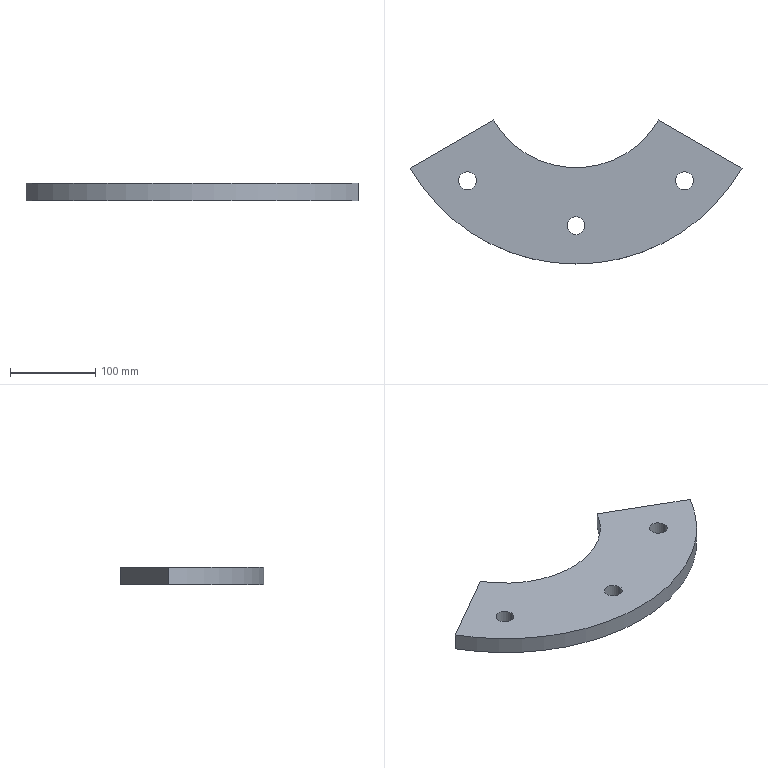Part | STEP file | Part 7 | 1 solid | 12 faces | box 389.711 x 169 x 20 mm | volume 776785 mm3 | cylinder 8 | plane 4 | commonest cylinder face diameters 21 x6 224 x1 450 x1
STEP:
#1=CARTESIAN_POINT('',(0.,0.,0.));
#2=DIRECTION('',(0.,0.,1.));
#3=DIRECTION('',(1.,0.,0.));
#4=AXIS2_PLACEMENT_3D('',#1,#2,#3);
#5=CARTESIAN_POINT('',(116.779,-127.279,20.));
#6=VERTEX_POINT('',#5);
#7=CARTESIAN_POINT('',(116.779,-127.279,0.));
#8=VERTEX_POINT('',#7);
#9=CARTESIAN_POINT('',(116.779,-127.279,20.));
#10=DIRECTION('',(0.,0.,-1.));
#11=VECTOR('',#10,1.);
#12=LINE('',#9,#11);
#13=CARTESIAN_POINT('',(127.279,-127.279,20.));
#14=DIRECTION('',(0.,0.,-1.));
#15=DIRECTION('',(-1.,0.,0.));
#16=AXIS2_PLACEMENT_3D('',#13,#14,#15);
#17=CYLINDRICAL_SURFACE('',#16,10.5);
#18=CARTESIAN_POINT('',(6.283,0.));
#19=DIRECTION('',(0.,1.));
#20=VECTOR('',#19,1.);
#21=LINE('',#18,#20);
#22=(GEOMETRIC_REPRESENTATION_CONTEXT(2)PARAMETRIC_REPRESENTATION_CONTEXT()REPRESENTATION_CONTEXT('',''));
#23=DEFINITIONAL_REPRESENTATION('',(#21),#22);
#24=PCURVE('',#17,#23);
#25=CARTESIAN_POINT('',(127.279,-127.279,20.));
#26=DIRECTION('',(0.,0.,-1.));
#27=DIRECTION('',(-1.,0.,0.));
#28=AXIS2_PLACEMENT_3D('',#25,#26,#27);
#29=CYLINDRICAL_SURFACE('',#28,10.5);
#30=CARTESIAN_POINT('',(0.,0.));
#31=DIRECTION('',(0.,1.));
#32=VECTOR('',#31,1.);
#33=LINE('',#30,#32);
#34=(GEOMETRIC_REPRESENTATION_CONTEXT(2)PARAMETRIC_REPRESENTATION_CONTEXT()REPRESENTATION_CONTEXT('',''));
#35=DEFINITIONAL_REPRESENTATION('',(#33),#34);
#36=PCURVE('',#29,#35);
#37=SURFACE_CURVE('',#12,(#24,#36),.PCURVE_S1.);
#38=EDGE_CURVE('',#6,#8,#37,.T.);
#39=ORIENTED_EDGE('',*,*,#38,.T.);
#40=CARTESIAN_POINT('',(137.779,-127.279,0.));
#41=VERTEX_POINT('',#40);
#42=CARTESIAN_POINT('',(127.279,-127.279,0.));
#43=DIRECTION('',(0.,0.,1.));
#44=DIRECTION('',(1.,0.,0.));
#45=AXIS2_PLACEMENT_3D('',#42,#43,#44);
#46=CIRCLE('',#45,10.5);
#47=CARTESIAN_POINT('',(9.425,20.));
#48=DIRECTION('',(-1.,0.));
#49=VECTOR('',#48,1.);
#50=LINE('',#47,#49);
#51=(GEOMETRIC_REPRESENTATION_CONTEXT(2)PARAMETRIC_REPRESENTATION_CONTEXT()REPRESENTATION_CONTEXT('',''));
#52=DEFINITIONAL_REPRESENTATION('',(#50),#51);
#53=PCURVE('',#17,#52);
#54=CARTESIAN_POINT('',(0.,0.,0.));
#55=DIRECTION('',(0.,0.,1.));
#56=DIRECTION('',(1.,0.,0.));
#57=AXIS2_PLACEMENT_3D('',#54,#55,#56);
#58=PLANE('',#57);
#59=CARTESIAN_POINT('',(127.279,-127.279));
#60=DIRECTION('',(1.,0.));
#61=AXIS2_PLACEMENT_2D('',#59,#60);
#62=CIRCLE('',#61,10.5);
#63=(GEOMETRIC_REPRESENTATION_CONTEXT(2)PARAMETRIC_REPRESENTATION_CONTEXT()REPRESENTATION_CONTEXT('',''));
#64=DEFINITIONAL_REPRESENTATION('',(#62),#63);
#65=PCURVE('',#58,#64);
#66=SURFACE_CURVE('',#46,(#53,#65),.PCURVE_S1.);
#67=EDGE_CURVE('',#8,#41,#66,.T.);
#68=ORIENTED_EDGE('',*,*,#67,.T.);
#69=CARTESIAN_POINT('',(137.779,-127.279,20.));
#70=VERTEX_POINT('',#69);
#71=CARTESIAN_POINT('',(137.779,-127.279,20.));
#72=DIRECTION('',(0.,0.,-1.));
#73=VECTOR('',#72,1.);
#74=LINE('',#71,#73);
#75=CARTESIAN_POINT('',(3.142,0.));
#76=DIRECTION('',(0.,1.));
#77=VECTOR('',#76,1.);
#78=LINE('',#75,#77);
#79=(GEOMETRIC_REPRESENTATION_CONTEXT(2)PARAMETRIC_REPRESENTATION_CONTEXT()REPRESENTATION_CONTEXT('',''));
#80=DEFINITIONAL_REPRESENTATION('',(#78),#79);
#81=PCURVE('',#17,#80);
#82=CARTESIAN_POINT('',(3.142,0.));
#83=DIRECTION('',(0.,1.));
#84=VECTOR('',#83,1.);
#85=LINE('',#82,#84);
#86=(GEOMETRIC_REPRESENTATION_CONTEXT(2)PARAMETRIC_REPRESENTATION_CONTEXT()REPRESENTATION_CONTEXT('',''));
#87=DEFINITIONAL_REPRESENTATION('',(#85),#86);
#88=PCURVE('',#29,#87);
#89=SURFACE_CURVE('',#74,(#81,#88),.PCURVE_S1.);
#90=EDGE_CURVE('',#70,#41,#89,.T.);
#91=ORIENTED_EDGE('',*,*,#90,.F.);
#92=CARTESIAN_POINT('',(127.279,-127.279,20.));
#93=DIRECTION('',(0.,0.,1.));
#94=DIRECTION('',(1.,0.,0.));
#95=AXIS2_PLACEMENT_3D('',#92,#93,#94);
#96=CIRCLE('',#95,10.5);
#97=CARTESIAN_POINT('',(9.425,0.));
#98=DIRECTION('',(-1.,0.));
#99=VECTOR('',#98,1.);
#100=LINE('',#97,#99);
#101=(GEOMETRIC_REPRESENTATION_CONTEXT(2)PARAMETRIC_REPRESENTATION_CONTEXT()REPRESENTATION_CONTEXT('',''));
#102=DEFINITIONAL_REPRESENTATION('',(#100),#101);
#103=PCURVE('',#17,#102);
#104=CARTESIAN_POINT('',(0.,0.,20.));
#105=DIRECTION('',(0.,0.,1.));
#106=DIRECTION('',(1.,0.,0.));
#107=AXIS2_PLACEMENT_3D('',#104,#105,#106);
#108=PLANE('',#107);
#109=CARTESIAN_POINT('',(127.279,-127.279));
#110=DIRECTION('',(1.,0.));
#111=AXIS2_PLACEMENT_2D('',#109,#110);
#112=CIRCLE('',#111,10.5);
#113=(GEOMETRIC_REPRESENTATION_CONTEXT(2)PARAMETRIC_REPRESENTATION_CONTEXT()REPRESENTATION_CONTEXT('',''));
#114=DEFINITIONAL_REPRESENTATION('',(#112),#113);
#115=PCURVE('',#108,#114);
#116=SURFACE_CURVE('',#96,(#103,#115),.PCURVE_S1.);
#117=EDGE_CURVE('',#6,#70,#116,.T.);
#118=ORIENTED_EDGE('',*,*,#117,.F.);
#119=EDGE_LOOP('',(#39,#68,#91,#118));
#120=FACE_BOUND('',#119,.F.);
#121=ADVANCED_FACE('',(#120),#17,.F.);
#122=CARTESIAN_POINT('',(-10.5,-180.,20.));
#123=VERTEX_POINT('',#122);
#124=CARTESIAN_POINT('',(-10.5,-180.,0.));
#125=VERTEX_POINT('',#124);
#126=CARTESIAN_POINT('',(-10.5,-180.,20.));
#127=DIRECTION('',(0.,0.,-1.));
#128=VECTOR('',#127,1.);
#129=LINE('',#126,#128);
#130=CARTESIAN_POINT('',(0.,-180.,20.));
#131=DIRECTION('',(0.,0.,-1.));
#132=DIRECTION('',(-1.,0.,0.));
#133=AXIS2_PLACEMENT_3D('',#130,#131,#132);
#134=CYLINDRICAL_SURFACE('',#133,10.5);
#135=CARTESIAN_POINT('',(6.283,0.));
#136=DIRECTION('',(0.,1.));
#137=VECTOR('',#136,1.);
#138=LINE('',#135,#137);
#139=(GEOMETRIC_REPRESENTATION_CONTEXT(2)PARAMETRIC_REPRESENTATION_CONTEXT()REPRESENTATION_CONTEXT('',''));
#140=DEFINITIONAL_REPRESENTATION('',(#138),#139);
#141=PCURVE('',#134,#140);
#142=CARTESIAN_POINT('',(0.,-180.,20.));
#143=DIRECTION('',(0.,0.,-1.));
#144=DIRECTION('',(-1.,0.,0.));
#145=AXIS2_PLACEMENT_3D('',#142,#143,#144);
#146=CYLINDRICAL_SURFACE('',#145,10.5);
#147=CARTESIAN_POINT('',(0.,0.));
#148=DIRECTION('',(0.,1.));
#149=VECTOR('',#148,1.);
#150=LINE('',#147,#149);
#151=(GEOMETRIC_REPRESENTATION_CONTEXT(2)PARAMETRIC_REPRESENTATION_CONTEXT()REPRESENTATION_CONTEXT('',''));
#152=DEFINITIONAL_REPRESENTATION('',(#150),#151);
#153=PCURVE('',#146,#152);
#154=SURFACE_CURVE('',#129,(#141,#153),.PCURVE_S1.);
#155=EDGE_CURVE('',#123,#125,#154,.T.);
#156=ORIENTED_EDGE('',*,*,#155,.T.);
#157=CARTESIAN_POINT('',(10.5,-180.,0.));
#158=VERTEX_POINT('',#157);
#159=CARTESIAN_POINT('',(0.,-180.,0.));
#160=DIRECTION('',(0.,0.,1.));
#161=DIRECTION('',(1.,0.,0.));
#162=AXIS2_PLACEMENT_3D('',#159,#160,#161);
#163=CIRCLE('',#162,10.5);
#164=CARTESIAN_POINT('',(9.425,20.));
#165=DIRECTION('',(-1.,0.));
#166=VECTOR('',#165,1.);
#167=LINE('',#164,#166);
#168=(GEOMETRIC_REPRESENTATION_CONTEXT(2)PARAMETRIC_REPRESENTATION_CONTEXT()REPRESENTATION_CONTEXT('',''));
#169=DEFINITIONAL_REPRESENTATION('',(#167),#168);
#170=PCURVE('',#134,#169);
#171=CARTESIAN_POINT('',(0.,-180.));
#172=DIRECTION('',(1.,0.));
#173=AXIS2_PLACEMENT_2D('',#171,#172);
#174=CIRCLE('',#173,10.5);
#175=(GEOMETRIC_REPRESENTATION_CONTEXT(2)PARAMETRIC_REPRESENTATION_CONTEXT()REPRESENTATION_CONTEXT('',''));
#176=DEFINITIONAL_REPRESENTATION('',(#174),#175);
#177=PCURVE('',#58,#176);
#178=SURFACE_CURVE('',#163,(#170,#177),.PCURVE_S1.);
#179=EDGE_CURVE('',#125,#158,#178,.T.);
#180=ORIENTED_EDGE('',*,*,#179,.T.);
#181=CARTESIAN_POINT('',(10.5,-180.,20.));
#182=VERTEX_POINT('',#181);
#183=CARTESIAN_POINT('',(10.5,-180.,20.));
#184=DIRECTION('',(0.,0.,-1.));
#185=VECTOR('',#184,1.);
#186=LINE('',#183,#185);
#187=CARTESIAN_POINT('',(3.142,0.));
#188=DIRECTION('',(0.,1.));
#189=VECTOR('',#188,1.);
#190=LINE('',#187,#189);
#191=(GEOMETRIC_REPRESENTATION_CONTEXT(2)PARAMETRIC_REPRESENTATION_CONTEXT()REPRESENTATION_CONTEXT('',''));
#192=DEFINITIONAL_REPRESENTATION('',(#190),#191);
#193=PCURVE('',#134,#192);
#194=CARTESIAN_POINT('',(3.142,0.));
#195=DIRECTION('',(0.,1.));
#196=VECTOR('',#195,1.);
#197=LINE('',#194,#196);
#198=(GEOMETRIC_REPRESENTATION_CONTEXT(2)PARAMETRIC_REPRESENTATION_CONTEXT()REPRESENTATION_CONTEXT('',''));
#199=DEFINITIONAL_REPRESENTATION('',(#197),#198);
#200=PCURVE('',#146,#199);
#201=SURFACE_CURVE('',#186,(#193,#200),.PCURVE_S1.);
#202=EDGE_CURVE('',#182,#158,#201,.T.);
#203=ORIENTED_EDGE('',*,*,#202,.F.);
#204=CARTESIAN_POINT('',(0.,-180.,20.));
#205=DIRECTION('',(0.,0.,1.));
#206=DIRECTION('',(1.,0.,0.));
#207=AXIS2_PLACEMENT_3D('',#204,#205,#206);
#208=CIRCLE('',#207,10.5);
#209=CARTESIAN_POINT('',(9.425,0.));
#210=DIRECTION('',(-1.,0.));
#211=VECTOR('',#210,1.);
#212=LINE('',#209,#211);
#213=(GEOMETRIC_REPRESENTATION_CONTEXT(2)PARAMETRIC_REPRESENTATION_CONTEXT()REPRESENTATION_CONTEXT('',''));
#214=DEFINITIONAL_REPRESENTATION('',(#212),#213);
#215=PCURVE('',#134,#214);
#216=CARTESIAN_POINT('',(0.,-180.));
#217=DIRECTION('',(1.,0.));
#218=AXIS2_PLACEMENT_2D('',#216,#217);
#219=CIRCLE('',#218,10.5);
#220=(GEOMETRIC_REPRESENTATION_CONTEXT(2)PARAMETRIC_REPRESENTATION_CONTEXT()REPRESENTATION_CONTEXT('',''));
#221=DEFINITIONAL_REPRESENTATION('',(#219),#220);
#222=PCURVE('',#108,#221);
#223=SURFACE_CURVE('',#208,(#215,#222),.PCURVE_S1.);
#224=EDGE_CURVE('',#123,#182,#223,.T.);
#225=ORIENTED_EDGE('',*,*,#224,.F.);
#226=EDGE_LOOP('',(#156,#180,#203,#225));
#227=FACE_BOUND('',#226,.F.);
#228=ADVANCED_FACE('',(#227),#134,.F.);
#229=CARTESIAN_POINT('',(-137.779,-127.279,20.));
#230=VERTEX_POINT('',#229);
#231=CARTESIAN_POINT('',(-137.779,-127.279,0.));
#232=VERTEX_POINT('',#231);
#233=CARTESIAN_POINT('',(-137.779,-127.279,20.));
#234=DIRECTION('',(0.,0.,-1.));
#235=VECTOR('',#234,1.);
#236=LINE('',#233,#235);
#237=CARTESIAN_POINT('',(-127.279,-127.279,20.));
#238=DIRECTION('',(0.,0.,-1.));
#239=DIRECTION('',(-1.,0.,0.));
#240=AXIS2_PLACEMENT_3D('',#237,#238,#239);
#241=CYLINDRICAL_SURFACE('',#240,10.5);
#242=CARTESIAN_POINT('',(6.283,0.));
#243=DIRECTION('',(0.,1.));
#244=VECTOR('',#243,1.);
#245=LINE('',#242,#244);
#246=(GEOMETRIC_REPRESENTATION_CONTEXT(2)PARAMETRIC_REPRESENTATION_CONTEXT()REPRESENTATION_CONTEXT('',''));
#247=DEFINITIONAL_REPRESENTATION('',(#245),#246);
#248=PCURVE('',#241,#247);
#249=CARTESIAN_POINT('',(-127.279,-127.279,20.));
#250=DIRECTION('',(0.,0.,-1.));
#251=DIRECTION('',(-1.,0.,0.));
#252=AXIS2_PLACEMENT_3D('',#249,#250,#251);
#253=CYLINDRICAL_SURFACE('',#252,10.5);
#254=CARTESIAN_POINT('',(0.,0.));
#255=DIRECTION('',(0.,1.));
#256=VECTOR('',#255,1.);
#257=LINE('',#254,#256);
#258=(GEOMETRIC_REPRESENTATION_CONTEXT(2)PARAMETRIC_REPRESENTATION_CONTEXT()REPRESENTATION_CONTEXT('',''));
#259=DEFINITIONAL_REPRESENTATION('',(#257),#258);
#260=PCURVE('',#253,#259);
#261=SURFACE_CURVE('',#236,(#248,#260),.PCURVE_S1.);
#262=EDGE_CURVE('',#230,#232,#261,.T.);
#263=ORIENTED_EDGE('',*,*,#262,.T.);
#264=CARTESIAN_POINT('',(-116.779,-127.279,0.));
#265=VERTEX_POINT('',#264);
#266=CARTESIAN_POINT('',(-127.279,-127.279,0.));
#267=DIRECTION('',(0.,0.,1.));
#268=DIRECTION('',(1.,0.,0.));
#269=AXIS2_PLACEMENT_3D('',#266,#267,#268);
#270=CIRCLE('',#269,10.5);
#271=CARTESIAN_POINT('',(9.425,20.));
#272=DIRECTION('',(-1.,0.));
#273=VECTOR('',#272,1.);
#274=LINE('',#271,#273);
#275=(GEOMETRIC_REPRESENTATION_CONTEXT(2)PARAMETRIC_REPRESENTATION_CONTEXT()REPRESENTATION_CONTEXT('',''));
#276=DEFINITIONAL_REPRESENTATION('',(#274),#275);
#277=PCURVE('',#241,#276);
#278=CARTESIAN_POINT('',(-127.279,-127.279));
#279=DIRECTION('',(1.,0.));
#280=AXIS2_PLACEMENT_2D('',#278,#279);
#281=CIRCLE('',#280,10.5);
#282=(GEOMETRIC_REPRESENTATION_CONTEXT(2)PARAMETRIC_REPRESENTATION_CONTEXT()REPRESENTATION_CONTEXT('',''));
#283=DEFINITIONAL_REPRESENTATION('',(#281),#282);
#284=PCURVE('',#58,#283);
#285=SURFACE_CURVE('',#270,(#277,#284),.PCURVE_S1.);
#286=EDGE_CURVE('',#232,#265,#285,.T.);
#287=ORIENTED_EDGE('',*,*,#286,.T.);
#288=CARTESIAN_POINT('',(-116.779,-127.279,20.));
#289=VERTEX_POINT('',#288);
#290=CARTESIAN_POINT('',(-116.779,-127.279,20.));
#291=DIRECTION('',(0.,0.,-1.));
#292=VECTOR('',#291,1.);
#293=LINE('',#290,#292);
#294=CARTESIAN_POINT('',(3.142,0.));
#295=DIRECTION('',(0.,1.));
#296=VECTOR('',#295,1.);
#297=LINE('',#294,#296);
#298=(GEOMETRIC_REPRESENTATION_CONTEXT(2)PARAMETRIC_REPRESENTATION_CONTEXT()REPRESENTATION_CONTEXT('',''));
#299=DEFINITIONAL_REPRESENTATION('',(#297),#298);
#300=PCURVE('',#241,#299);
#301=CARTESIAN_POINT('',(3.142,0.));
#302=DIRECTION('',(0.,1.));
#303=VECTOR('',#302,1.);
#304=LINE('',#301,#303);
#305=(GEOMETRIC_REPRESENTATION_CONTEXT(2)PARAMETRIC_REPRESENTATION_CONTEXT()REPRESENTATION_CONTEXT('',''));
#306=DEFINITIONAL_REPRESENTATION('',(#304),#305);
#307=PCURVE('',#253,#306);
#308=SURFACE_CURVE('',#293,(#300,#307),.PCURVE_S1.);
#309=EDGE_CURVE('',#289,#265,#308,.T.);
#310=ORIENTED_EDGE('',*,*,#309,.F.);
#311=CARTESIAN_POINT('',(-127.279,-127.279,20.));
#312=DIRECTION('',(0.,0.,1.));
#313=DIRECTION('',(1.,0.,0.));
#314=AXIS2_PLACEMENT_3D('',#311,#312,#313);
#315=CIRCLE('',#314,10.5);
#316=CARTESIAN_POINT('',(9.425,0.));
#317=DIRECTION('',(-1.,0.));
#318=VECTOR('',#317,1.);
#319=LINE('',#316,#318);
#320=(GEOMETRIC_REPRESENTATION_CONTEXT(2)PARAMETRIC_REPRESENTATION_CONTEXT()REPRESENTATION_CONTEXT('',''));
#321=DEFINITIONAL_REPRESENTATION('',(#319),#320);
#322=PCURVE('',#241,#321);
#323=CARTESIAN_POINT('',(-127.279,-127.279));
#324=DIRECTION('',(1.,0.));
#325=AXIS2_PLACEMENT_2D('',#323,#324);
#326=CIRCLE('',#325,10.5);
#327=(GEOMETRIC_REPRESENTATION_CONTEXT(2)PARAMETRIC_REPRESENTATION_CONTEXT()REPRESENTATION_CONTEXT('',''));
#328=DEFINITIONAL_REPRESENTATION('',(#326),#327);
#329=PCURVE('',#108,#328);
#330=SURFACE_CURVE('',#315,(#322,#329),.PCURVE_S1.);
#331=EDGE_CURVE('',#230,#289,#330,.T.);
#332=ORIENTED_EDGE('',*,*,#331,.F.);
#333=EDGE_LOOP('',(#263,#287,#310,#332));
#334=FACE_BOUND('',#333,.F.);
#335=ADVANCED_FACE('',(#334),#241,.F.);
#336=ORIENTED_EDGE('',*,*,#224,.F.);
#337=CARTESIAN_POINT('',(0.,-180.,20.));
#338=DIRECTION('',(0.,0.,1.));
#339=DIRECTION('',(1.,0.,0.));
#340=AXIS2_PLACEMENT_3D('',#337,#338,#339);
#341=CIRCLE('',#340,10.5);
#342=CARTESIAN_POINT('',(0.,-180.));
#343=DIRECTION('',(1.,0.));
#344=AXIS2_PLACEMENT_2D('',#342,#343);
#345=CIRCLE('',#344,10.5);
#346=(GEOMETRIC_REPRESENTATION_CONTEXT(2)PARAMETRIC_REPRESENTATION_CONTEXT()REPRESENTATION_CONTEXT('',''));
#347=DEFINITIONAL_REPRESENTATION('',(#345),#346);
#348=PCURVE('',#108,#347);
#349=CARTESIAN_POINT('',(3.142,0.));
#350=DIRECTION('',(-1.,0.));
#351=VECTOR('',#350,1.);
#352=LINE('',#349,#351);
#353=(GEOMETRIC_REPRESENTATION_CONTEXT(2)PARAMETRIC_REPRESENTATION_CONTEXT()REPRESENTATION_CONTEXT('',''));
#354=DEFINITIONAL_REPRESENTATION('',(#352),#353);
#355=PCURVE('',#146,#354);
#356=SURFACE_CURVE('',#341,(#348,#355),.PCURVE_S1.);
#357=EDGE_CURVE('',#182,#123,#356,.T.);
#358=ORIENTED_EDGE('',*,*,#357,.F.);
#359=EDGE_LOOP('',(#336,#358));
#360=FACE_BOUND('',#359,.T.);
#361=CARTESIAN_POINT('',(96.995,-56.,20.));
#362=VERTEX_POINT('',#361);
#363=CARTESIAN_POINT('',(-96.995,-56.,20.));
#364=VERTEX_POINT('',#363);
#365=CARTESIAN_POINT('',(0.,0.,20.));
#366=DIRECTION('',(0.,0.,-1.));
#367=DIRECTION('',(1.,0.,0.));
#368=AXIS2_PLACEMENT_3D('',#365,#366,#367);
#369=CIRCLE('',#368,112.);
#370=CARTESIAN_POINT('',(112.,0.));
#371=CARTESIAN_POINT('',(112.,-193.99));
#372=CARTESIAN_POINT('',(-56.,-96.995));
#373=CARTESIAN_POINT('',(-224.,0.));
#374=CARTESIAN_POINT('',(-56.,96.995));
#375=CARTESIAN_POINT('',(112.,193.99));
#376=CARTESIAN_POINT('',(112.,0.));
#377=(BOUNDED_CURVE()B_SPLINE_CURVE(2,(#370,#371,#372,#373,#374,#375,#376),.UNSPECIFIED.,.T.,.F.)B_SPLINE_CURVE_WITH_KNOTS((1,2,2,2,2,1),(-2.094,0.,2.094,4.189,6.283,8.378),.UNSPECIFIED.)CURVE()GEOMETRIC_REPRESENTATION_ITEM()RATIONAL_B_SPLINE_CURVE((1.,0.5,1.,0.5,1.,0.5,1.))REPRESENTATION_ITEM(''));
#378=(GEOMETRIC_REPRESENTATION_CONTEXT(2)PARAMETRIC_REPRESENTATION_CONTEXT()REPRESENTATION_CONTEXT('',''));
#379=DEFINITIONAL_REPRESENTATION('',(#377),#378);
#380=PCURVE('',#108,#379);
#381=CARTESIAN_POINT('',(0.,0.,20.));
#382=DIRECTION('',(0.,0.,-1.));
#383=DIRECTION('',(-1.,0.,0.));
#384=AXIS2_PLACEMENT_3D('',#381,#382,#383);
#385=CYLINDRICAL_SURFACE('',#384,112.);
#386=CARTESIAN_POINT('',(3.142,0.));
#387=DIRECTION('',(1.,0.));
#388=VECTOR('',#387,1.);
#389=LINE('',#386,#388);
#390=(GEOMETRIC_REPRESENTATION_CONTEXT(2)PARAMETRIC_REPRESENTATION_CONTEXT()REPRESENTATION_CONTEXT('',''));
#391=DEFINITIONAL_REPRESENTATION('',(#389),#390);
#392=PCURVE('',#385,#391);
#393=SURFACE_CURVE('',#369,(#380,#392),.PCURVE_S1.);
#394=EDGE_CURVE('',#362,#364,#393,.T.);
#395=ORIENTED_EDGE('',*,*,#394,.T.);
#396=CARTESIAN_POINT('',(-194.856,-112.5,20.));
#397=VERTEX_POINT('',#396);
#398=CARTESIAN_POINT('',(-96.995,-56.,20.));
#399=DIRECTION('',(-0.866,-0.5,0.));
#400=VECTOR('',#399,1.);
#401=LINE('',#398,#400);
#402=CARTESIAN_POINT('',(-96.995,-56.));
#403=DIRECTION('',(-0.866,-0.5));
#404=VECTOR('',#403,1.);
#405=LINE('',#402,#404);
#406=(GEOMETRIC_REPRESENTATION_CONTEXT(2)PARAMETRIC_REPRESENTATION_CONTEXT()REPRESENTATION_CONTEXT('',''));
#407=DEFINITIONAL_REPRESENTATION('',(#405),#406);
#408=PCURVE('',#108,#407);
#409=CARTESIAN_POINT('',(-97.211,-56.125,20.));
#410=DIRECTION('',(0.5,-0.866,0.));
#411=DIRECTION('',(0.866,0.5,0.));
#412=AXIS2_PLACEMENT_3D('',#409,#410,#411);
#413=PLANE('',#412);
#414=CARTESIAN_POINT('',(0.2497,0.));
#415=DIRECTION('',(-1.,0.));
#416=VECTOR('',#415,1.);
#417=LINE('',#414,#416);
#418=(GEOMETRIC_REPRESENTATION_CONTEXT(2)PARAMETRIC_REPRESENTATION_CONTEXT()REPRESENTATION_CONTEXT('',''));
#419=DEFINITIONAL_REPRESENTATION('',(#417),#418);
#420=PCURVE('',#413,#419);
#421=SURFACE_CURVE('',#401,(#408,#420),.PCURVE_S1.);
#422=EDGE_CURVE('',#364,#397,#421,.T.);
#423=ORIENTED_EDGE('',*,*,#422,.T.);
#424=CARTESIAN_POINT('',(194.856,-112.5,20.));
#425=VERTEX_POINT('',#424);
#426=CARTESIAN_POINT('',(0.,0.,20.));
#427=DIRECTION('',(0.,0.,1.));
#428=DIRECTION('',(1.,0.,0.));
#429=AXIS2_PLACEMENT_3D('',#426,#427,#428);
#430=CIRCLE('',#429,225.);
#431=CARTESIAN_POINT('',(0.,0.));
#432=DIRECTION('',(1.,0.));
#433=AXIS2_PLACEMENT_2D('',#431,#432);
#434=CIRCLE('',#433,225.);
#435=(GEOMETRIC_REPRESENTATION_CONTEXT(2)PARAMETRIC_REPRESENTATION_CONTEXT()REPRESENTATION_CONTEXT('',''));
#436=DEFINITIONAL_REPRESENTATION('',(#434),#435);
#437=PCURVE('',#108,#436);
#438=CARTESIAN_POINT('',(0.,0.,20.));
#439=DIRECTION('',(0.,0.,-1.));
#440=DIRECTION('',(-1.,0.,0.));
#441=AXIS2_PLACEMENT_3D('',#438,#439,#440);
#442=CYLINDRICAL_SURFACE('',#441,225.);
#443=CARTESIAN_POINT('',(9.425,0.));
#444=DIRECTION('',(-1.,0.));
#445=VECTOR('',#444,1.);
#446=LINE('',#443,#445);
#447=(GEOMETRIC_REPRESENTATION_CONTEXT(2)PARAMETRIC_REPRESENTATION_CONTEXT()REPRESENTATION_CONTEXT('',''));
#448=DEFINITIONAL_REPRESENTATION('',(#446),#447);
#449=PCURVE('',#442,#448);
#450=SURFACE_CURVE('',#430,(#437,#449),.PCURVE_S1.);
#451=EDGE_CURVE('',#397,#425,#450,.T.);
#452=ORIENTED_EDGE('',*,*,#451,.T.);
#453=CARTESIAN_POINT('',(194.856,-112.5,20.));
#454=DIRECTION('',(-0.866,0.5,0.));
#455=VECTOR('',#454,1.);
#456=LINE('',#453,#455);
#457=CARTESIAN_POINT('',(194.856,-112.5));
#458=DIRECTION('',(-0.866,0.5));
#459=VECTOR('',#458,1.);
#460=LINE('',#457,#459);
#461=(GEOMETRIC_REPRESENTATION_CONTEXT(2)PARAMETRIC_REPRESENTATION_CONTEXT()REPRESENTATION_CONTEXT('',''));
#462=DEFINITIONAL_REPRESENTATION('',(#460),#461);
#463=PCURVE('',#108,#462);
#464=CARTESIAN_POINT('',(97.211,-56.125,20.));
#465=DIRECTION('',(-0.5,-0.866,0.));
#466=DIRECTION('',(0.866,-0.5,0.));
#467=AXIS2_PLACEMENT_3D('',#464,#465,#466);
#468=PLANE('',#467);
#469=CARTESIAN_POINT('',(112.75,0.));
#470=DIRECTION('',(-1.,0.));
#471=VECTOR('',#470,1.);
#472=LINE('',#469,#471);
#473=(GEOMETRIC_REPRESENTATION_CONTEXT(2)PARAMETRIC_REPRESENTATION_CONTEXT()REPRESENTATION_CONTEXT('',''));
#474=DEFINITIONAL_REPRESENTATION('',(#472),#473);
#475=PCURVE('',#468,#474);
#476=SURFACE_CURVE('',#456,(#463,#475),.PCURVE_S1.);
#477=EDGE_CURVE('',#425,#362,#476,.T.);
#478=ORIENTED_EDGE('',*,*,#477,.T.);
#479=EDGE_LOOP('',(#395,#423,#452,#478));
#480=FACE_BOUND('',#479,.T.);
#481=ORIENTED_EDGE('',*,*,#331,.F.);
#482=CARTESIAN_POINT('',(-127.279,-127.279,20.));
#483=DIRECTION('',(0.,0.,1.));
#484=DIRECTION('',(1.,0.,0.));
#485=AXIS2_PLACEMENT_3D('',#482,#483,#484);
#486=CIRCLE('',#485,10.5);
#487=CARTESIAN_POINT('',(-127.279,-127.279));
#488=DIRECTION('',(1.,0.));
#489=AXIS2_PLACEMENT_2D('',#487,#488);
#490=CIRCLE('',#489,10.5);
#491=(GEOMETRIC_REPRESENTATION_CONTEXT(2)PARAMETRIC_REPRESENTATION_CONTEXT()REPRESENTATION_CONTEXT('',''));
#492=DEFINITIONAL_REPRESENTATION('',(#490),#491);
#493=PCURVE('',#108,#492);
#494=CARTESIAN_POINT('',(3.142,0.));
#495=DIRECTION('',(-1.,0.));
#496=VECTOR('',#495,1.);
#497=LINE('',#494,#496);
#498=(GEOMETRIC_REPRESENTATION_CONTEXT(2)PARAMETRIC_REPRESENTATION_CONTEXT()REPRESENTATION_CONTEXT('',''));
#499=DEFINITIONAL_REPRESENTATION('',(#497),#498);
#500=PCURVE('',#253,#499);
#501=SURFACE_CURVE('',#486,(#493,#500),.PCURVE_S1.);
#502=EDGE_CURVE('',#289,#230,#501,.T.);
#503=ORIENTED_EDGE('',*,*,#502,.F.);
#504=EDGE_LOOP('',(#481,#503));
#505=FACE_BOUND('',#504,.T.);
#506=ORIENTED_EDGE('',*,*,#117,.F.);
#507=CARTESIAN_POINT('',(127.279,-127.279,20.));
#508=DIRECTION('',(0.,0.,1.));
#509=DIRECTION('',(1.,0.,0.));
#510=AXIS2_PLACEMENT_3D('',#507,#508,#509);
#511=CIRCLE('',#510,10.5);
#512=CARTESIAN_POINT('',(127.279,-127.279));
#513=DIRECTION('',(1.,0.));
#514=AXIS2_PLACEMENT_2D('',#512,#513);
#515=CIRCLE('',#514,10.5);
#516=(GEOMETRIC_REPRESENTATION_CONTEXT(2)PARAMETRIC_REPRESENTATION_CONTEXT()REPRESENTATION_CONTEXT('',''));
#517=DEFINITIONAL_REPRESENTATION('',(#515),#516);
#518=PCURVE('',#108,#517);
#519=CARTESIAN_POINT('',(3.142,0.));
#520=DIRECTION('',(-1.,0.));
#521=VECTOR('',#520,1.);
#522=LINE('',#519,#521);
#523=(GEOMETRIC_REPRESENTATION_CONTEXT(2)PARAMETRIC_REPRESENTATION_CONTEXT()REPRESENTATION_CONTEXT('',''));
#524=DEFINITIONAL_REPRESENTATION('',(#522),#523);
#525=PCURVE('',#29,#524);
#526=SURFACE_CURVE('',#511,(#518,#525),.PCURVE_S1.);
#527=EDGE_CURVE('',#70,#6,#526,.T.);
#528=ORIENTED_EDGE('',*,*,#527,.F.);
#529=EDGE_LOOP('',(#506,#528));
#530=FACE_BOUND('',#529,.T.);
#531=ADVANCED_FACE('',(#360,#480,#505,#530),#108,.T.);
#532=ORIENTED_EDGE('',*,*,#179,.T.);
#533=CARTESIAN_POINT('',(0.,-180.,0.));
#534=DIRECTION('',(0.,0.,1.));
#535=DIRECTION('',(1.,0.,0.));
#536=AXIS2_PLACEMENT_3D('',#533,#534,#535);
#537=CIRCLE('',#536,10.5);
#538=CARTESIAN_POINT('',(0.,-180.));
#539=DIRECTION('',(1.,0.));
#540=AXIS2_PLACEMENT_2D('',#538,#539);
#541=CIRCLE('',#540,10.5);
#542=(GEOMETRIC_REPRESENTATION_CONTEXT(2)PARAMETRIC_REPRESENTATION_CONTEXT()REPRESENTATION_CONTEXT('',''));
#543=DEFINITIONAL_REPRESENTATION('',(#541),#542);
#544=PCURVE('',#58,#543);
#545=CARTESIAN_POINT('',(3.142,20.));
#546=DIRECTION('',(-1.,0.));
#547=VECTOR('',#546,1.);
#548=LINE('',#545,#547);
#549=(GEOMETRIC_REPRESENTATION_CONTEXT(2)PARAMETRIC_REPRESENTATION_CONTEXT()REPRESENTATION_CONTEXT('',''));
#550=DEFINITIONAL_REPRESENTATION('',(#548),#549);
#551=PCURVE('',#146,#550);
#552=SURFACE_CURVE('',#537,(#544,#551),.PCURVE_S1.);
#553=EDGE_CURVE('',#158,#125,#552,.T.);
#554=ORIENTED_EDGE('',*,*,#553,.T.);
#555=EDGE_LOOP('',(#532,#554));
#556=FACE_BOUND('',#555,.T.);
#557=CARTESIAN_POINT('',(96.995,-56.,0.));
#558=VERTEX_POINT('',#557);
#559=CARTESIAN_POINT('',(-96.995,-56.,0.));
#560=VERTEX_POINT('',#559);
#561=CARTESIAN_POINT('',(0.,0.,0.));
#562=DIRECTION('',(0.,0.,-1.));
#563=DIRECTION('',(1.,0.,0.));
#564=AXIS2_PLACEMENT_3D('',#561,#562,#563);
#565=CIRCLE('',#564,112.);
#566=CARTESIAN_POINT('',(112.,0.));
#567=CARTESIAN_POINT('',(112.,-193.99));
#568=CARTESIAN_POINT('',(-56.,-96.995));
#569=CARTESIAN_POINT('',(-224.,0.));
#570=CARTESIAN_POINT('',(-56.,96.995));
#571=CARTESIAN_POINT('',(112.,193.99));
#572=CARTESIAN_POINT('',(112.,0.));
#573=(BOUNDED_CURVE()B_SPLINE_CURVE(2,(#566,#567,#568,#569,#570,#571,#572),.UNSPECIFIED.,.T.,.F.)B_SPLINE_CURVE_WITH_KNOTS((1,2,2,2,2,1),(-2.094,0.,2.094,4.189,6.283,8.378),.UNSPECIFIED.)CURVE()GEOMETRIC_REPRESENTATION_ITEM()RATIONAL_B_SPLINE_CURVE((1.,0.5,1.,0.5,1.,0.5,1.))REPRESENTATION_ITEM(''));
#574=(GEOMETRIC_REPRESENTATION_CONTEXT(2)PARAMETRIC_REPRESENTATION_CONTEXT()REPRESENTATION_CONTEXT('',''));
#575=DEFINITIONAL_REPRESENTATION('',(#573),#574);
#576=PCURVE('',#58,#575);
#577=CARTESIAN_POINT('',(3.142,20.));
#578=DIRECTION('',(1.,0.));
#579=VECTOR('',#578,1.);
#580=LINE('',#577,#579);
#581=(GEOMETRIC_REPRESENTATION_CONTEXT(2)PARAMETRIC_REPRESENTATION_CONTEXT()REPRESENTATION_CONTEXT('',''));
#582=DEFINITIONAL_REPRESENTATION('',(#580),#581);
#583=PCURVE('',#385,#582);
#584=SURFACE_CURVE('',#565,(#576,#583),.PCURVE_S1.);
#585=EDGE_CURVE('',#558,#560,#584,.T.);
#586=ORIENTED_EDGE('',*,*,#585,.F.);
#587=CARTESIAN_POINT('',(194.856,-112.5,0.));
#588=VERTEX_POINT('',#587);
#589=CARTESIAN_POINT('',(97.211,-56.125,0.));
#590=DIRECTION('',(-0.866,0.5,0.));
#591=VECTOR('',#590,1.);
#592=LINE('',#589,#591);
#593=CARTESIAN_POINT('',(97.211,-56.125));
#594=DIRECTION('',(-0.866,0.5));
#595=VECTOR('',#594,1.);
#596=LINE('',#593,#595);
#597=(GEOMETRIC_REPRESENTATION_CONTEXT(2)PARAMETRIC_REPRESENTATION_CONTEXT()REPRESENTATION_CONTEXT('',''));
#598=DEFINITIONAL_REPRESENTATION('',(#596),#597);
#599=PCURVE('',#58,#598);
#600=CARTESIAN_POINT('',(0.,-20.));
#601=DIRECTION('',(-1.,0.));
#602=VECTOR('',#601,1.);
#603=LINE('',#600,#602);
#604=(GEOMETRIC_REPRESENTATION_CONTEXT(2)PARAMETRIC_REPRESENTATION_CONTEXT()REPRESENTATION_CONTEXT('',''));
#605=DEFINITIONAL_REPRESENTATION('',(#603),#604);
#606=PCURVE('',#468,#605);
#607=SURFACE_CURVE('',#592,(#599,#606),.PCURVE_S1.);
#608=EDGE_CURVE('',#588,#558,#607,.T.);
#609=ORIENTED_EDGE('',*,*,#608,.F.);
#610=CARTESIAN_POINT('',(-194.856,-112.5,0.));
#611=VERTEX_POINT('',#610);
#612=CARTESIAN_POINT('',(0.,0.,0.));
#613=DIRECTION('',(0.,0.,1.));
#614=DIRECTION('',(1.,0.,0.));
#615=AXIS2_PLACEMENT_3D('',#612,#613,#614);
#616=CIRCLE('',#615,225.);
#617=CARTESIAN_POINT('',(0.,0.));
#618=DIRECTION('',(1.,0.));
#619=AXIS2_PLACEMENT_2D('',#617,#618);
#620=CIRCLE('',#619,225.);
#621=(GEOMETRIC_REPRESENTATION_CONTEXT(2)PARAMETRIC_REPRESENTATION_CONTEXT()REPRESENTATION_CONTEXT('',''));
#622=DEFINITIONAL_REPRESENTATION('',(#620),#621);
#623=PCURVE('',#58,#622);
#624=CARTESIAN_POINT('',(9.425,20.));
#625=DIRECTION('',(-1.,0.));
#626=VECTOR('',#625,1.);
#627=LINE('',#624,#626);
#628=(GEOMETRIC_REPRESENTATION_CONTEXT(2)PARAMETRIC_REPRESENTATION_CONTEXT()REPRESENTATION_CONTEXT('',''));
#629=DEFINITIONAL_REPRESENTATION('',(#627),#628);
#630=PCURVE('',#442,#629);
#631=SURFACE_CURVE('',#616,(#623,#630),.PCURVE_S1.);
#632=EDGE_CURVE('',#611,#588,#631,.T.);
#633=ORIENTED_EDGE('',*,*,#632,.F.);
#634=CARTESIAN_POINT('',(-97.211,-56.125,0.));
#635=DIRECTION('',(-0.866,-0.5,0.));
#636=VECTOR('',#635,1.);
#637=LINE('',#634,#636);
#638=CARTESIAN_POINT('',(-97.211,-56.125));
#639=DIRECTION('',(-0.866,-0.5));
#640=VECTOR('',#639,1.);
#641=LINE('',#638,#640);
#642=(GEOMETRIC_REPRESENTATION_CONTEXT(2)PARAMETRIC_REPRESENTATION_CONTEXT()REPRESENTATION_CONTEXT('',''));
#643=DEFINITIONAL_REPRESENTATION('',(#641),#642);
#644=PCURVE('',#58,#643);
#645=CARTESIAN_POINT('',(0.,-20.));
#646=DIRECTION('',(-1.,0.));
#647=VECTOR('',#646,1.);
#648=LINE('',#645,#647);
#649=(GEOMETRIC_REPRESENTATION_CONTEXT(2)PARAMETRIC_REPRESENTATION_CONTEXT()REPRESENTATION_CONTEXT('',''));
#650=DEFINITIONAL_REPRESENTATION('',(#648),#649);
#651=PCURVE('',#413,#650);
#652=SURFACE_CURVE('',#637,(#644,#651),.PCURVE_S1.);
#653=EDGE_CURVE('',#560,#611,#652,.T.);
#654=ORIENTED_EDGE('',*,*,#653,.F.);
#655=EDGE_LOOP('',(#586,#609,#633,#654));
#656=FACE_BOUND('',#655,.T.);
#657=ORIENTED_EDGE('',*,*,#286,.T.);
#658=CARTESIAN_POINT('',(-127.279,-127.279,0.));
#659=DIRECTION('',(0.,0.,1.));
#660=DIRECTION('',(1.,0.,0.));
#661=AXIS2_PLACEMENT_3D('',#658,#659,#660);
#662=CIRCLE('',#661,10.5);
#663=CARTESIAN_POINT('',(-127.279,-127.279));
#664=DIRECTION('',(1.,0.));
#665=AXIS2_PLACEMENT_2D('',#663,#664);
#666=CIRCLE('',#665,10.5);
#667=(GEOMETRIC_REPRESENTATION_CONTEXT(2)PARAMETRIC_REPRESENTATION_CONTEXT()REPRESENTATION_CONTEXT('',''));
#668=DEFINITIONAL_REPRESENTATION('',(#666),#667);
#669=PCURVE('',#58,#668);
#670=CARTESIAN_POINT('',(3.142,20.));
#671=DIRECTION('',(-1.,0.));
#672=VECTOR('',#671,1.);
#673=LINE('',#670,#672);
#674=(GEOMETRIC_REPRESENTATION_CONTEXT(2)PARAMETRIC_REPRESENTATION_CONTEXT()REPRESENTATION_CONTEXT('',''));
#675=DEFINITIONAL_REPRESENTATION('',(#673),#674);
#676=PCURVE('',#253,#675);
#677=SURFACE_CURVE('',#662,(#669,#676),.PCURVE_S1.);
#678=EDGE_CURVE('',#265,#232,#677,.T.);
#679=ORIENTED_EDGE('',*,*,#678,.T.);
#680=EDGE_LOOP('',(#657,#679));
#681=FACE_BOUND('',#680,.T.);
#682=ORIENTED_EDGE('',*,*,#67,.T.);
#683=CARTESIAN_POINT('',(127.279,-127.279,0.));
#684=DIRECTION('',(0.,0.,1.));
#685=DIRECTION('',(1.,0.,0.));
#686=AXIS2_PLACEMENT_3D('',#683,#684,#685);
#687=CIRCLE('',#686,10.5);
#688=CARTESIAN_POINT('',(127.279,-127.279));
#689=DIRECTION('',(1.,0.));
#690=AXIS2_PLACEMENT_2D('',#688,#689);
#691=CIRCLE('',#690,10.5);
#692=(GEOMETRIC_REPRESENTATION_CONTEXT(2)PARAMETRIC_REPRESENTATION_CONTEXT()REPRESENTATION_CONTEXT('',''));
#693=DEFINITIONAL_REPRESENTATION('',(#691),#692);
#694=PCURVE('',#58,#693);
#695=CARTESIAN_POINT('',(3.142,20.));
#696=DIRECTION('',(-1.,0.));
#697=VECTOR('',#696,1.);
#698=LINE('',#695,#697);
#699=(GEOMETRIC_REPRESENTATION_CONTEXT(2)PARAMETRIC_REPRESENTATION_CONTEXT()REPRESENTATION_CONTEXT('',''));
#700=DEFINITIONAL_REPRESENTATION('',(#698),#699);
#701=PCURVE('',#29,#700);
#702=SURFACE_CURVE('',#687,(#694,#701),.PCURVE_S1.);
#703=EDGE_CURVE('',#41,#8,#702,.T.);
#704=ORIENTED_EDGE('',*,*,#703,.T.);
#705=EDGE_LOOP('',(#682,#704));
#706=FACE_BOUND('',#705,.T.);
#707=ADVANCED_FACE('',(#556,#656,#681,#706),#58,.F.);
#708=CARTESIAN_POINT('',(96.995,-56.,20.));
#709=DIRECTION('',(0.,0.,-1.));
#710=VECTOR('',#709,1.);
#711=LINE('',#708,#710);
#712=CARTESIAN_POINT('',(3.665,0.));
#713=DIRECTION('',(0.,1.));
#714=VECTOR('',#713,1.);
#715=LINE('',#712,#714);
#716=(GEOMETRIC_REPRESENTATION_CONTEXT(2)PARAMETRIC_REPRESENTATION_CONTEXT()REPRESENTATION_CONTEXT('',''));
#717=DEFINITIONAL_REPRESENTATION('',(#715),#716);
#718=PCURVE('',#385,#717);
#719=CARTESIAN_POINT('',(-0.2497,0.));
#720=DIRECTION('',(0.,-1.));
#721=VECTOR('',#720,1.);
#722=LINE('',#719,#721);
#723=(GEOMETRIC_REPRESENTATION_CONTEXT(2)PARAMETRIC_REPRESENTATION_CONTEXT()REPRESENTATION_CONTEXT('',''));
#724=DEFINITIONAL_REPRESENTATION('',(#722),#723);
#725=PCURVE('',#468,#724);
#726=SURFACE_CURVE('',#711,(#718,#725),.PCURVE_S1.);
#727=EDGE_CURVE('',#362,#558,#726,.T.);
#728=ORIENTED_EDGE('',*,*,#727,.F.);
#729=ORIENTED_EDGE('',*,*,#394,.T.);
#730=CARTESIAN_POINT('',(-96.995,-56.,20.));
#731=DIRECTION('',(0.,0.,-1.));
#732=VECTOR('',#731,1.);
#733=LINE('',#730,#732);
#734=CARTESIAN_POINT('',(5.76,0.));
#735=DIRECTION('',(0.,1.));
#736=VECTOR('',#735,1.);
#737=LINE('',#734,#736);
#738=(GEOMETRIC_REPRESENTATION_CONTEXT(2)PARAMETRIC_REPRESENTATION_CONTEXT()REPRESENTATION_CONTEXT('',''));
#739=DEFINITIONAL_REPRESENTATION('',(#737),#738);
#740=PCURVE('',#385,#739);
#741=CARTESIAN_POINT('',(0.2497,0.));
#742=DIRECTION('',(0.,-1.));
#743=VECTOR('',#742,1.);
#744=LINE('',#741,#743);
#745=(GEOMETRIC_REPRESENTATION_CONTEXT(2)PARAMETRIC_REPRESENTATION_CONTEXT()REPRESENTATION_CONTEXT('',''));
#746=DEFINITIONAL_REPRESENTATION('',(#744),#745);
#747=PCURVE('',#413,#746);
#748=SURFACE_CURVE('',#733,(#740,#747),.PCURVE_S1.);
#749=EDGE_CURVE('',#364,#560,#748,.T.);
#750=ORIENTED_EDGE('',*,*,#749,.T.);
#751=ORIENTED_EDGE('',*,*,#585,.F.);
#752=EDGE_LOOP('',(#728,#729,#750,#751));
#753=FACE_BOUND('',#752,.F.);
#754=ADVANCED_FACE('',(#753),#385,.F.);
#755=ORIENTED_EDGE('',*,*,#653,.T.);
#756=CARTESIAN_POINT('',(-194.856,-112.5,20.));
#757=DIRECTION('',(0.,0.,-1.));
#758=VECTOR('',#757,1.);
#759=LINE('',#756,#758);
#760=CARTESIAN_POINT('',(-112.75,0.));
#761=DIRECTION('',(0.,-1.));
#762=VECTOR('',#761,1.);
#763=LINE('',#760,#762);
#764=(GEOMETRIC_REPRESENTATION_CONTEXT(2)PARAMETRIC_REPRESENTATION_CONTEXT()REPRESENTATION_CONTEXT('',''));
#765=DEFINITIONAL_REPRESENTATION('',(#763),#764);
#766=PCURVE('',#413,#765);
#767=CARTESIAN_POINT('',(5.76,0.));
#768=DIRECTION('',(0.,1.));
#769=VECTOR('',#768,1.);
#770=LINE('',#767,#769);
#771=(GEOMETRIC_REPRESENTATION_CONTEXT(2)PARAMETRIC_REPRESENTATION_CONTEXT()REPRESENTATION_CONTEXT('',''));
#772=DEFINITIONAL_REPRESENTATION('',(#770),#771);
#773=PCURVE('',#442,#772);
#774=SURFACE_CURVE('',#759,(#766,#773),.PCURVE_S1.);
#775=EDGE_CURVE('',#397,#611,#774,.T.);
#776=ORIENTED_EDGE('',*,*,#775,.F.);
#777=ORIENTED_EDGE('',*,*,#422,.F.);
#778=ORIENTED_EDGE('',*,*,#749,.T.);
#779=EDGE_LOOP('',(#755,#776,#777,#778));
#780=FACE_BOUND('',#779,.T.);
#781=ADVANCED_FACE('',(#780),#413,.F.);
#782=ORIENTED_EDGE('',*,*,#632,.T.);
#783=CARTESIAN_POINT('',(194.856,-112.5,20.));
#784=DIRECTION('',(0.,0.,-1.));
#785=VECTOR('',#784,1.);
#786=LINE('',#783,#785);
#787=CARTESIAN_POINT('',(3.665,0.));
#788=DIRECTION('',(0.,1.));
#789=VECTOR('',#788,1.);
#790=LINE('',#787,#789);
#791=(GEOMETRIC_REPRESENTATION_CONTEXT(2)PARAMETRIC_REPRESENTATION_CONTEXT()REPRESENTATION_CONTEXT('',''));
#792=DEFINITIONAL_REPRESENTATION('',(#790),#791);
#793=PCURVE('',#442,#792);
#794=CARTESIAN_POINT('',(112.75,0.));
#795=DIRECTION('',(0.,-1.));
#796=VECTOR('',#795,1.);
#797=LINE('',#794,#796);
#798=(GEOMETRIC_REPRESENTATION_CONTEXT(2)PARAMETRIC_REPRESENTATION_CONTEXT()REPRESENTATION_CONTEXT('',''));
#799=DEFINITIONAL_REPRESENTATION('',(#797),#798);
#800=PCURVE('',#468,#799);
#801=SURFACE_CURVE('',#786,(#793,#800),.PCURVE_S1.);
#802=EDGE_CURVE('',#425,#588,#801,.T.);
#803=ORIENTED_EDGE('',*,*,#802,.F.);
#804=ORIENTED_EDGE('',*,*,#451,.F.);
#805=ORIENTED_EDGE('',*,*,#775,.T.);
#806=EDGE_LOOP('',(#782,#803,#804,#805));
#807=FACE_BOUND('',#806,.T.);
#808=ADVANCED_FACE('',(#807),#442,.T.);
#809=ORIENTED_EDGE('',*,*,#608,.T.);
#810=ORIENTED_EDGE('',*,*,#727,.F.);
#811=ORIENTED_EDGE('',*,*,#477,.F.);
#812=ORIENTED_EDGE('',*,*,#802,.T.);
#813=EDGE_LOOP('',(#809,#810,#811,#812));
#814=FACE_BOUND('',#813,.T.);
#815=ADVANCED_FACE('',(#814),#468,.F.);
#816=ORIENTED_EDGE('',*,*,#678,.T.);
#817=ORIENTED_EDGE('',*,*,#262,.F.);
#818=ORIENTED_EDGE('',*,*,#502,.F.);
#819=ORIENTED_EDGE('',*,*,#309,.T.);
#820=EDGE_LOOP('',(#816,#817,#818,#819));
#821=FACE_BOUND('',#820,.F.);
#822=ADVANCED_FACE('',(#821),#253,.F.);
#823=ORIENTED_EDGE('',*,*,#553,.T.);
#824=ORIENTED_EDGE('',*,*,#155,.F.);
#825=ORIENTED_EDGE('',*,*,#357,.F.);
#826=ORIENTED_EDGE('',*,*,#202,.T.);
#827=EDGE_LOOP('',(#823,#824,#825,#826));
#828=FACE_BOUND('',#827,.F.);
#829=ADVANCED_FACE('',(#828),#146,.F.);
#830=ORIENTED_EDGE('',*,*,#703,.T.);
#831=ORIENTED_EDGE('',*,*,#38,.F.);
#832=ORIENTED_EDGE('',*,*,#527,.F.);
#833=ORIENTED_EDGE('',*,*,#90,.T.);
#834=EDGE_LOOP('',(#830,#831,#832,#833));
#835=FACE_BOUND('',#834,.F.);
#836=ADVANCED_FACE('',(#835),#29,.F.);
#837=CLOSED_SHELL('',(#121,#228,#335,#531,#707,#754,#781,#808,#815,#822,#829,#836));
#838=MANIFOLD_SOLID_BREP('',#837);
#839=(LENGTH_UNIT()NAMED_UNIT(*)SI_UNIT(.MILLI.,.METRE.));
#840=UNCERTAINTY_MEASURE_WITH_UNIT(LENGTH_MEASURE(0.0000001),#839,'','');
#841=(NAMED_UNIT(*)PLANE_ANGLE_UNIT()SI_UNIT($,.RADIAN.));
#842=(NAMED_UNIT(*)SI_UNIT($,.STERADIAN.)SOLID_ANGLE_UNIT());
#843=(GEOMETRIC_REPRESENTATION_CONTEXT(3)GLOBAL_UNCERTAINTY_ASSIGNED_CONTEXT((#840))GLOBAL_UNIT_ASSIGNED_CONTEXT((#839,#841,#842))REPRESENTATION_CONTEXT('',''));
#844=ADVANCED_BREP_SHAPE_REPRESENTATION('',(#4,#838),#843);